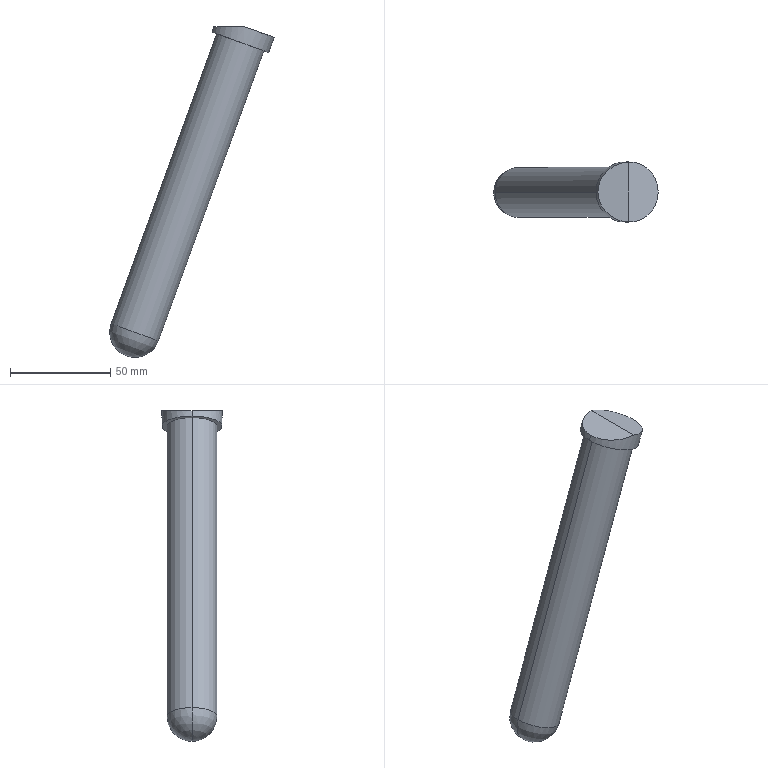Part | Creo | 1 solid | 9 faces | box 81.921 x 30 x 164.735 mm | volume 84487 mm3 | cylinder 4 | plane 3 | sphere 2 | commonest cylinder face diameters 25 x2 30 x2
STEP:
#1=CARTESIAN_POINT('',(-206.527,129.995,32.639));
#2=VERTEX_POINT('',#1);
#3=CARTESIAN_POINT('',(-221.255,144.98,38.));
#4=VERTEX_POINT('',#3);
#5=CARTESIAN_POINT('',(-220.623,129.995,37.77));
#6=DIRECTION('',(0.342,0.,0.9397));
#7=DIRECTION('',(0.9397,-0.000000002,-0.342));
#8=AXIS2_PLACEMENT_3D('',#5,#6,#7);
#9=CIRCLE('',#8,15.);
#10=EDGE_CURVE('',#2,#4,#9,.T.);
#11=ORIENTED_EDGE('',*,*,#10,.T.);
#12=CARTESIAN_POINT('',(-236.501,129.995,38.));
#13=VERTEX_POINT('',#12);
#14=CARTESIAN_POINT('',(-221.255,144.98,38.));
#15=CARTESIAN_POINT('',(-222.314,144.935,38.));
#16=CARTESIAN_POINT('',(-224.372,144.654,38.));
#17=CARTESIAN_POINT('',(-227.336,143.673,38.));
#18=CARTESIAN_POINT('',(-230.006,142.186,38.));
#19=CARTESIAN_POINT('',(-232.297,140.276,38.));
#20=CARTESIAN_POINT('',(-234.171,137.973,38.));
#21=CARTESIAN_POINT('',(-235.511,135.441,38.));
#22=CARTESIAN_POINT('',(-236.32,132.757,38.));
#23=CARTESIAN_POINT('',(-236.501,130.926,38.));
#24=CARTESIAN_POINT('',(-236.501,129.995,38.));
#25=B_SPLINE_CURVE_WITH_KNOTS('',3,(#14,#15,#16,#17,#18,#19,#20,#21,#22,#23,#24),.UNSPECIFIED.,.F.,.F.,(4,1,1,1,1,1,1,1,4),(0.,0.125,0.25,0.375,0.5,0.625,0.75,0.875,1.),.UNSPECIFIED.);
#26=EDGE_CURVE('',#4,#13,#25,.T.);
#27=ORIENTED_EDGE('',*,*,#26,.T.);
#28=CARTESIAN_POINT('',(-237.454,129.995,35.382));
#29=VERTEX_POINT('',#28);
#30=CARTESIAN_POINT('',(-236.501,129.995,38.));
#31=DIRECTION('',(-0.342,0.000000007,-0.9397));
#32=VECTOR('',#31,2.786);
#33=LINE('',#30,#32);
#34=EDGE_CURVE('',#13,#29,#33,.T.);
#35=ORIENTED_EDGE('',*,*,#34,.T.);
#36=CARTESIAN_POINT('',(-209.263,129.995,25.122));
#37=VERTEX_POINT('',#36);
#38=CARTESIAN_POINT('',(-223.359,129.995,30.252));
#39=DIRECTION('',(-0.342,0.,-0.9397));
#40=DIRECTION('',(-0.9397,0.,0.342));
#41=AXIS2_PLACEMENT_3D('',#38,#39,#40);
#42=CIRCLE('',#41,15.);
#43=EDGE_CURVE('',#29,#37,#42,.T.);
#44=ORIENTED_EDGE('',*,*,#43,.T.);
#45=CARTESIAN_POINT('',(-206.527,129.995,32.639));
#46=DIRECTION('',(-0.342,0.000000001,-0.9397));
#47=VECTOR('',#46,8.);
#48=LINE('',#45,#47);
#49=EDGE_CURVE('',#2,#37,#48,.T.);
#50=ORIENTED_EDGE('',*,*,#49,.F.);
#51=EDGE_LOOP('',(#11,#27,#35,#44,#50));
#52=FACE_OUTER_BOUND('',#51,.F.);
#53=CARTESIAN_POINT('',(-217.527,129.995,46.274));
#54=DIRECTION('',(-0.342,0.,-0.9397));
#55=DIRECTION('',(-0.9397,0.,0.342));
#56=AXIS2_PLACEMENT_3D('',#53,#54,#55);
#57=CYLINDRICAL_SURFACE('',#56,15.);
#58=ADVANCED_FACE('',(#52),#57,.T.);
#59=ORIENTED_EDGE('',*,*,#10,.F.);
#60=CARTESIAN_POINT('',(-221.255,115.01,38.));
#61=VERTEX_POINT('',#60);
#62=CARTESIAN_POINT('',(-220.623,129.995,37.77));
#63=DIRECTION('',(0.342,0.,0.9397));
#64=DIRECTION('',(-0.0422,-0.999,0.01536));
#65=AXIS2_PLACEMENT_3D('',#62,#63,#64);
#66=CIRCLE('',#65,15.);
#67=EDGE_CURVE('',#61,#2,#66,.T.);
#68=ORIENTED_EDGE('',*,*,#67,.F.);
#69=CARTESIAN_POINT('',(-221.255,144.98,38.));
#70=DIRECTION('',(0.,-1.,0.));
#71=VECTOR('',#70,29.97);
#72=LINE('',#69,#71);
#73=EDGE_CURVE('',#4,#61,#72,.T.);
#74=ORIENTED_EDGE('',*,*,#73,.F.);
#75=EDGE_LOOP('',(#59,#68,#74));
#76=FACE_OUTER_BOUND('',#75,.F.);
#77=CARTESIAN_POINT('',(-220.623,129.995,37.77));
#78=DIRECTION('',(-0.342,0.,-0.9397));
#79=DIRECTION('',(-0.9397,0.,0.342));
#80=AXIS2_PLACEMENT_3D('',#77,#78,#79);
#81=PLANE('',#80);
#82=ADVANCED_FACE('',(#76),#81,.F.);
#83=ORIENTED_EDGE('',*,*,#67,.T.);
#84=ORIENTED_EDGE('',*,*,#49,.T.);
#85=CARTESIAN_POINT('',(-223.359,129.995,30.252));
#86=DIRECTION('',(-0.342,0.,-0.9397));
#87=DIRECTION('',(0.9397,0.,-0.342));
#88=AXIS2_PLACEMENT_3D('',#85,#86,#87);
#89=CIRCLE('',#88,15.);
#90=EDGE_CURVE('',#37,#29,#89,.T.);
#91=ORIENTED_EDGE('',*,*,#90,.T.);
#92=ORIENTED_EDGE('',*,*,#34,.F.);
#93=CARTESIAN_POINT('',(-236.501,129.995,38.));
#94=CARTESIAN_POINT('',(-236.501,129.158,38.));
#95=CARTESIAN_POINT('',(-236.354,127.512,38.));
#96=CARTESIAN_POINT('',(-235.71,125.119,38.));
#97=CARTESIAN_POINT('',(-234.655,122.845,38.));
#98=CARTESIAN_POINT('',(-233.189,120.731,38.));
#99=CARTESIAN_POINT('',(-231.353,118.865,38.));
#100=CARTESIAN_POINT('',(-229.198,117.307,38.));
#101=CARTESIAN_POINT('',(-226.755,116.097,38.));
#102=CARTESIAN_POINT('',(-224.08,115.29,38.));
#103=CARTESIAN_POINT('',(-222.215,115.051,38.));
#104=CARTESIAN_POINT('',(-221.255,115.01,38.));
#105=B_SPLINE_CURVE_WITH_KNOTS('',3,(#93,#94,#95,#96,#97,#98,#99,#100,#101,#102,#103,#104),.UNSPECIFIED.,.F.,.F.,(4,1,1,1,1,1,1,1,1,4),(0.,0.1111,0.2222,0.3333,0.4444,0.5556,0.6667,0.7778,0.8889,1.),.UNSPECIFIED.);
#106=EDGE_CURVE('',#13,#61,#105,.T.);
#107=ORIENTED_EDGE('',*,*,#106,.T.);
#108=EDGE_LOOP('',(#83,#84,#91,#92,#107));
#109=FACE_OUTER_BOUND('',#108,.F.);
#110=CARTESIAN_POINT('',(-217.527,129.995,46.274));
#111=DIRECTION('',(-0.342,0.,-0.9397));
#112=DIRECTION('',(-0.9397,0.,0.342));
#113=AXIS2_PLACEMENT_3D('',#110,#111,#112);
#114=CYLINDRICAL_SURFACE('',#113,15.);
#115=ADVANCED_FACE('',(#109),#114,.T.);
#116=ORIENTED_EDGE('',*,*,#90,.F.);
#117=ORIENTED_EDGE('',*,*,#43,.F.);
#118=EDGE_LOOP('',(#116,#117));
#119=FACE_OUTER_BOUND('',#118,.F.);
#120=CARTESIAN_POINT('',(-211.613,129.995,25.977));
#121=VERTEX_POINT('',#120);
#122=CARTESIAN_POINT('',(-235.105,129.995,34.527));
#123=VERTEX_POINT('',#122);
#124=CARTESIAN_POINT('',(-223.359,129.995,30.252));
#125=DIRECTION('',(0.342,0.,0.9397));
#126=DIRECTION('',(0.9397,0.,-0.342));
#127=AXIS2_PLACEMENT_3D('',#124,#125,#126);
#128=CIRCLE('',#127,12.5);
#129=EDGE_CURVE('',#121,#123,#128,.T.);
#130=ORIENTED_EDGE('',*,*,#129,.F.);
#131=CARTESIAN_POINT('',(-223.359,129.995,30.252));
#132=DIRECTION('',(0.342,0.,0.9397));
#133=DIRECTION('',(-0.9397,0.,0.342));
#134=AXIS2_PLACEMENT_3D('',#131,#132,#133);
#135=CIRCLE('',#134,12.5);
#136=EDGE_CURVE('',#123,#121,#135,.T.);
#137=ORIENTED_EDGE('',*,*,#136,.F.);
#138=EDGE_LOOP('',(#130,#137));
#139=FACE_BOUND('',#138,.F.);
#140=CARTESIAN_POINT('',(-223.359,129.995,30.252));
#141=DIRECTION('',(-0.342,0.,-0.9397));
#142=DIRECTION('',(-0.9397,0.,0.342));
#143=AXIS2_PLACEMENT_3D('',#140,#141,#142);
#144=PLANE('',#143);
#145=ADVANCED_FACE('',(#119,#139),#144,.T.);
#146=ORIENTED_EDGE('',*,*,#129,.T.);
#147=CARTESIAN_POINT('',(-287.694,129.995,-109.96));
#148=VERTEX_POINT('',#147);
#149=CARTESIAN_POINT('',(-235.105,129.995,34.527));
#150=DIRECTION('',(-0.342,0.,-0.9397));
#151=VECTOR('',#150,153.76);
#152=LINE('',#149,#151);
#153=EDGE_CURVE('',#123,#148,#152,.T.);
#154=ORIENTED_EDGE('',*,*,#153,.T.);
#155=CARTESIAN_POINT('',(-264.202,129.995,-118.51));
#156=VERTEX_POINT('',#155);
#157=CARTESIAN_POINT('',(-275.948,129.995,-114.235));
#158=DIRECTION('',(-0.342,0.,-0.9397));
#159=DIRECTION('',(-0.9397,0.,0.342));
#160=AXIS2_PLACEMENT_3D('',#157,#158,#159);
#161=CIRCLE('',#160,12.5);
#162=EDGE_CURVE('',#148,#156,#161,.T.);
#163=ORIENTED_EDGE('',*,*,#162,.T.);
#164=CARTESIAN_POINT('',(-211.613,129.995,25.977));
#165=DIRECTION('',(-0.342,0.,-0.9397));
#166=VECTOR('',#165,153.76);
#167=LINE('',#164,#166);
#168=EDGE_CURVE('',#121,#156,#167,.T.);
#169=ORIENTED_EDGE('',*,*,#168,.F.);
#170=EDGE_LOOP('',(#146,#154,#163,#169));
#171=FACE_OUTER_BOUND('',#170,.F.);
#172=CARTESIAN_POINT('',(-211.802,129.995,62.004));
#173=DIRECTION('',(-0.342,0.,-0.9397));
#174=DIRECTION('',(-0.9397,0.,0.342));
#175=AXIS2_PLACEMENT_3D('',#172,#173,#174);
#176=CYLINDRICAL_SURFACE('',#175,12.5);
#177=ADVANCED_FACE('',(#171),#176,.T.);
#178=ORIENTED_EDGE('',*,*,#136,.T.);
#179=ORIENTED_EDGE('',*,*,#168,.T.);
#180=CARTESIAN_POINT('',(-275.948,129.995,-114.235));
#181=DIRECTION('',(-0.342,0.,-0.9397));
#182=DIRECTION('',(0.9397,0.,-0.342));
#183=AXIS2_PLACEMENT_3D('',#180,#181,#182);
#184=CIRCLE('',#183,12.5);
#185=EDGE_CURVE('',#156,#148,#184,.T.);
#186=ORIENTED_EDGE('',*,*,#185,.T.);
#187=ORIENTED_EDGE('',*,*,#153,.F.);
#188=EDGE_LOOP('',(#178,#179,#186,#187));
#189=FACE_OUTER_BOUND('',#188,.F.);
#190=CARTESIAN_POINT('',(-211.802,129.995,62.004));
#191=DIRECTION('',(-0.342,0.,-0.9397));
#192=DIRECTION('',(-0.9397,0.,0.342));
#193=AXIS2_PLACEMENT_3D('',#190,#191,#192);
#194=CYLINDRICAL_SURFACE('',#193,12.5);
#195=ADVANCED_FACE('',(#189),#194,.T.);
#196=ORIENTED_EDGE('',*,*,#185,.F.);
#197=CARTESIAN_POINT('',(-280.223,129.995,-125.981));
#198=VERTEX_POINT('',#197);
#199=CARTESIAN_POINT('',(-275.948,129.995,-114.235));
#200=DIRECTION('',(0.,1.,0.));
#201=DIRECTION('',(0.9397,0.,-0.342));
#202=AXIS2_PLACEMENT_3D('',#199,#200,#201);
#203=CIRCLE('',#202,12.5);
#204=EDGE_CURVE('',#156,#198,#203,.T.);
#205=ORIENTED_EDGE('',*,*,#204,.T.);
#206=CARTESIAN_POINT('',(-275.948,129.995,-114.235));
#207=DIRECTION('',(0.,-1.,0.));
#208=DIRECTION('',(-0.9397,0.,0.342));
#209=AXIS2_PLACEMENT_3D('',#206,#207,#208);
#210=CIRCLE('',#209,12.5);
#211=EDGE_CURVE('',#148,#198,#210,.T.);
#212=ORIENTED_EDGE('',*,*,#211,.F.);
#213=EDGE_LOOP('',(#196,#205,#212));
#214=FACE_OUTER_BOUND('',#213,.F.);
#215=CARTESIAN_POINT('',(-275.948,129.995,-114.235));
#216=DIRECTION('',(-0.342,0.,-0.9397));
#217=DIRECTION('',(-0.9397,0.,0.342));
#218=AXIS2_PLACEMENT_3D('',#215,#216,#217);
#219=SPHERICAL_SURFACE('',#218,12.5);
#220=ADVANCED_FACE('',(#214),#219,.T.);
#221=ORIENTED_EDGE('',*,*,#162,.F.);
#222=ORIENTED_EDGE('',*,*,#211,.T.);
#223=ORIENTED_EDGE('',*,*,#204,.F.);
#224=EDGE_LOOP('',(#221,#222,#223));
#225=FACE_OUTER_BOUND('',#224,.F.);
#226=CARTESIAN_POINT('',(-275.948,129.995,-114.235));
#227=DIRECTION('',(-0.342,0.,-0.9397));
#228=DIRECTION('',(-0.9397,0.,0.342));
#229=AXIS2_PLACEMENT_3D('',#226,#227,#228);
#230=SPHERICAL_SURFACE('',#229,12.5);
#231=ADVANCED_FACE('',(#225),#230,.T.);
#232=ORIENTED_EDGE('',*,*,#106,.F.);
#233=ORIENTED_EDGE('',*,*,#26,.F.);
#234=ORIENTED_EDGE('',*,*,#73,.T.);
#235=EDGE_LOOP('',(#232,#233,#234));
#236=FACE_OUTER_BOUND('',#235,.F.);
#237=CARTESIAN_POINT('',(-225.833,-493.939,38.));
#238=DIRECTION('',(0.,0.,1.));
#239=DIRECTION('',(0.,1.,0.));
#240=AXIS2_PLACEMENT_3D('',#237,#238,#239);
#241=PLANE('',#240);
#242=ADVANCED_FACE('',(#236),#241,.T.);
#243=CLOSED_SHELL('',(#58,#82,#115,#145,#177,#195,#220,#231,#242));
#244=MANIFOLD_SOLID_BREP('',#243);
#245=(LENGTH_UNIT()NAMED_UNIT(*)SI_UNIT(.MILLI.,.METRE.));
#246=UNCERTAINTY_MEASURE_WITH_UNIT(LENGTH_MEASURE(0.01907),#245,'','');
#247=(NAMED_UNIT(*)PLANE_ANGLE_UNIT()SI_UNIT($,.RADIAN.));
#248=PLANE_ANGLE_MEASURE_WITH_UNIT(PLANE_ANGLE_MEASURE(0.01745),#247);
#249=(CONVERSION_BASED_UNIT('DEGREE',#248)NAMED_UNIT(*)PLANE_ANGLE_UNIT());
#250=(NAMED_UNIT(*)SI_UNIT($,.STERADIAN.)SOLID_ANGLE_UNIT());
#251=(GEOMETRIC_REPRESENTATION_CONTEXT(3)GLOBAL_UNCERTAINTY_ASSIGNED_CONTEXT((#246))GLOBAL_UNIT_ASSIGNED_CONTEXT((#245,#249,#250))REPRESENTATION_CONTEXT('',''));
#252=ADVANCED_BREP_SHAPE_REPRESENTATION('',(#244),#251);